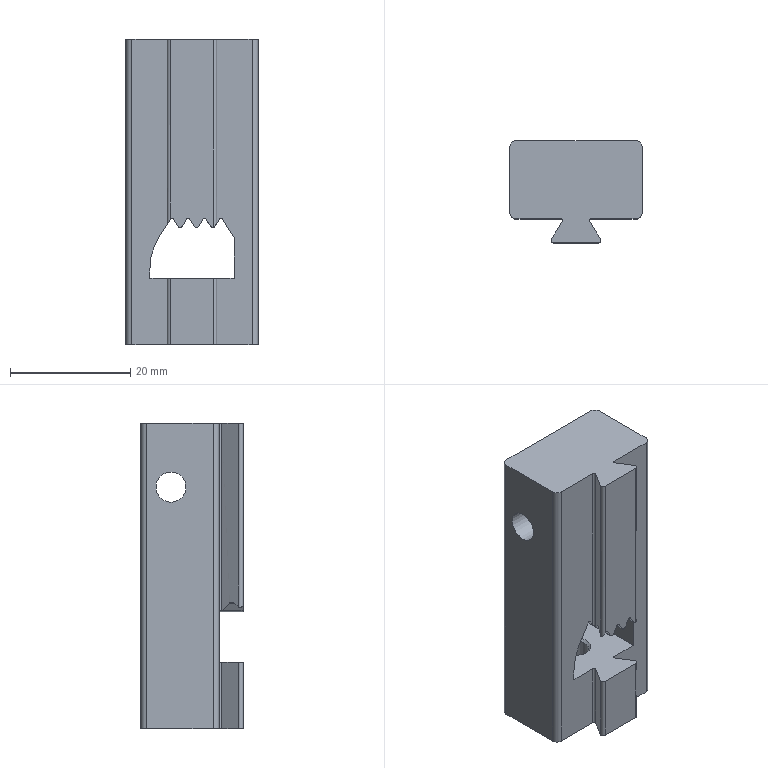Part | STEP file | 1 solid | 54 faces | box 22 x 17 x 50.8 mm | volume 13403 mm3 | plane 28 | cylinder 24 | cone 2 | commonest cylinder face diameters 0.62 x5 0.6 x4 0.78 x4 1 x4 2 x4 4.2 x1